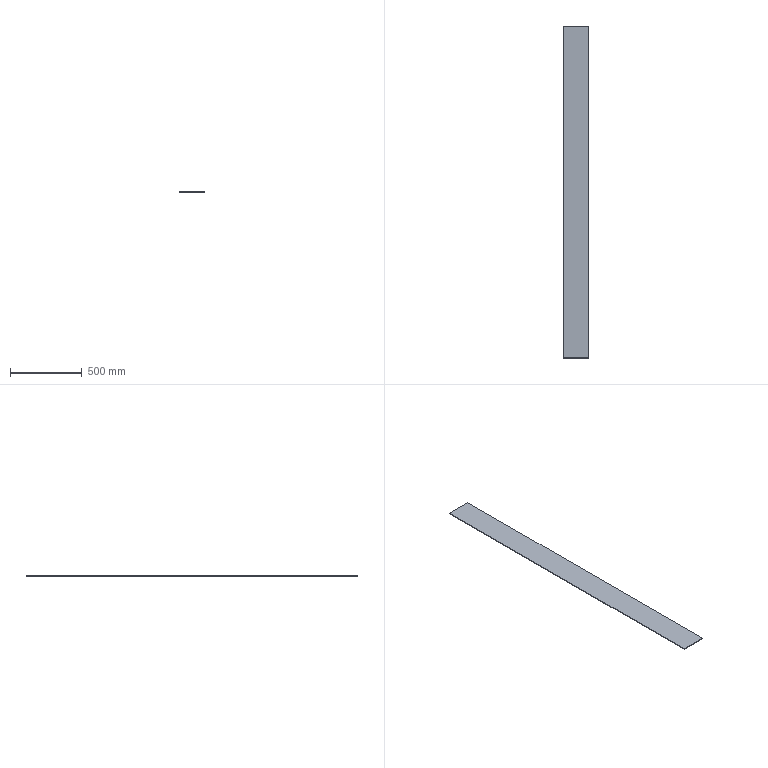Part | SolidWorks | features Extrusion 1, HoleWzd 1 | 1 solid | 6 faces | box 180 x 2310 x 5 mm | volume 2079000 mm3 | plane 6
STEP:
#1=CARTESIAN_POINT('',(90.,-1155.,0.));
#2=VERTEX_POINT('',#1);
#3=CARTESIAN_POINT('',(90.,1155.,0.));
#4=VERTEX_POINT('',#3);
#5=CARTESIAN_POINT('',(90.,1155.,0.));
#6=DIRECTION('',(0.,1.,0.));
#7=VECTOR('',#6,1000.);
#8=LINE('',#5,#7);
#9=EDGE_CURVE('',#2,#4,#8,.T.);
#10=ORIENTED_EDGE('',*,*,#9,.T.);
#11=CARTESIAN_POINT('',(90.,1155.,5.));
#12=VERTEX_POINT('',#11);
#13=CARTESIAN_POINT('',(90.,1155.,5.));
#14=DIRECTION('',(0.,0.,-1.));
#15=VECTOR('',#14,1000.);
#16=LINE('',#13,#15);
#17=EDGE_CURVE('',#12,#4,#16,.T.);
#18=ORIENTED_EDGE('',*,*,#17,.F.);
#19=CARTESIAN_POINT('',(90.,-1155.,5.));
#20=VERTEX_POINT('',#19);
#21=CARTESIAN_POINT('',(90.,1155.,5.));
#22=DIRECTION('',(0.,1.,0.));
#23=VECTOR('',#22,1000.);
#24=LINE('',#21,#23);
#25=EDGE_CURVE('',#20,#12,#24,.T.);
#26=ORIENTED_EDGE('',*,*,#25,.F.);
#27=CARTESIAN_POINT('',(90.,-1155.,5.));
#28=DIRECTION('',(0.,0.,-1.));
#29=VECTOR('',#28,1000.);
#30=LINE('',#27,#29);
#31=EDGE_CURVE('',#20,#2,#30,.T.);
#32=ORIENTED_EDGE('',*,*,#31,.T.);
#33=EDGE_LOOP('',(#10,#18,#26,#32));
#34=FACE_OUTER_BOUND('',#33,.T.);
#35=CARTESIAN_POINT('',(90.,1155.,5.));
#36=DIRECTION('',(-1.,0.,0.));
#37=DIRECTION('',(0.,-1.,0.));
#38=AXIS2_PLACEMENT_3D('',#35,#36,#37);
#39=PLANE('',#38);
#40=ADVANCED_FACE('',(#34),#39,.F.);
#41=CARTESIAN_POINT('',(-90.,1155.,0.));
#42=VERTEX_POINT('',#41);
#43=CARTESIAN_POINT('',(-90.,1155.,0.));
#44=DIRECTION('',(-1.,0.,0.));
#45=VECTOR('',#44,1000.);
#46=LINE('',#43,#45);
#47=EDGE_CURVE('',#4,#42,#46,.T.);
#48=ORIENTED_EDGE('',*,*,#47,.T.);
#49=CARTESIAN_POINT('',(-90.,1155.,5.));
#50=VERTEX_POINT('',#49);
#51=CARTESIAN_POINT('',(-90.,1155.,5.));
#52=DIRECTION('',(0.,0.,-1.));
#53=VECTOR('',#52,1000.);
#54=LINE('',#51,#53);
#55=EDGE_CURVE('',#50,#42,#54,.T.);
#56=ORIENTED_EDGE('',*,*,#55,.F.);
#57=CARTESIAN_POINT('',(-90.,1155.,5.));
#58=DIRECTION('',(-1.,0.,0.));
#59=VECTOR('',#58,1000.);
#60=LINE('',#57,#59);
#61=EDGE_CURVE('',#12,#50,#60,.T.);
#62=ORIENTED_EDGE('',*,*,#61,.F.);
#63=ORIENTED_EDGE('',*,*,#17,.T.);
#64=EDGE_LOOP('',(#48,#56,#62,#63));
#65=FACE_OUTER_BOUND('',#64,.T.);
#66=CARTESIAN_POINT('',(-90.,1155.,5.));
#67=DIRECTION('',(0.,-1.,0.));
#68=DIRECTION('',(0.,0.,-1.));
#69=AXIS2_PLACEMENT_3D('',#66,#67,#68);
#70=PLANE('',#69);
#71=ADVANCED_FACE('',(#65),#70,.F.);
#72=CARTESIAN_POINT('',(-90.,-1155.,0.));
#73=VERTEX_POINT('',#72);
#74=CARTESIAN_POINT('',(-90.,1155.,0.));
#75=DIRECTION('',(0.,-1.,0.));
#76=VECTOR('',#75,1000.);
#77=LINE('',#74,#76);
#78=EDGE_CURVE('',#42,#73,#77,.T.);
#79=ORIENTED_EDGE('',*,*,#78,.T.);
#80=CARTESIAN_POINT('',(-90.,-1155.,5.));
#81=VERTEX_POINT('',#80);
#82=CARTESIAN_POINT('',(-90.,-1155.,5.));
#83=DIRECTION('',(0.,0.,-1.));
#84=VECTOR('',#83,1000.);
#85=LINE('',#82,#84);
#86=EDGE_CURVE('',#81,#73,#85,.T.);
#87=ORIENTED_EDGE('',*,*,#86,.F.);
#88=CARTESIAN_POINT('',(-90.,1155.,5.));
#89=DIRECTION('',(0.,-1.,0.));
#90=VECTOR('',#89,1000.);
#91=LINE('',#88,#90);
#92=EDGE_CURVE('',#50,#81,#91,.T.);
#93=ORIENTED_EDGE('',*,*,#92,.F.);
#94=ORIENTED_EDGE('',*,*,#55,.T.);
#95=EDGE_LOOP('',(#79,#87,#93,#94));
#96=FACE_OUTER_BOUND('',#95,.T.);
#97=CARTESIAN_POINT('',(-90.,1155.,5.));
#98=DIRECTION('',(1.,0.,0.));
#99=DIRECTION('',(0.,1.,0.));
#100=AXIS2_PLACEMENT_3D('',#97,#98,#99);
#101=PLANE('',#100);
#102=ADVANCED_FACE('',(#96),#101,.F.);
#103=CARTESIAN_POINT('',(-90.,-1155.,0.));
#104=DIRECTION('',(1.,0.,0.));
#105=VECTOR('',#104,1000.);
#106=LINE('',#103,#105);
#107=EDGE_CURVE('',#73,#2,#106,.T.);
#108=ORIENTED_EDGE('',*,*,#107,.T.);
#109=ORIENTED_EDGE('',*,*,#31,.F.);
#110=CARTESIAN_POINT('',(-90.,-1155.,5.));
#111=DIRECTION('',(1.,0.,0.));
#112=VECTOR('',#111,1000.);
#113=LINE('',#110,#112);
#114=EDGE_CURVE('',#81,#20,#113,.T.);
#115=ORIENTED_EDGE('',*,*,#114,.F.);
#116=ORIENTED_EDGE('',*,*,#86,.T.);
#117=EDGE_LOOP('',(#108,#109,#115,#116));
#118=FACE_OUTER_BOUND('',#117,.T.);
#119=CARTESIAN_POINT('',(-90.,-1155.,5.));
#120=DIRECTION('',(0.,1.,0.));
#121=DIRECTION('',(0.,0.,1.));
#122=AXIS2_PLACEMENT_3D('',#119,#120,#121);
#123=PLANE('',#122);
#124=ADVANCED_FACE('',(#118),#123,.F.);
#125=ORIENTED_EDGE('',*,*,#25,.T.);
#126=ORIENTED_EDGE('',*,*,#61,.T.);
#127=ORIENTED_EDGE('',*,*,#92,.T.);
#128=ORIENTED_EDGE('',*,*,#114,.T.);
#129=EDGE_LOOP('',(#125,#126,#127,#128));
#130=FACE_OUTER_BOUND('',#129,.T.);
#131=CARTESIAN_POINT('',(0.,0.,5.));
#132=DIRECTION('',(0.,0.,1.));
#133=DIRECTION('',(1.,0.,0.));
#134=AXIS2_PLACEMENT_3D('',#131,#132,#133);
#135=PLANE('',#134);
#136=ADVANCED_FACE('',(#130),#135,.T.);
#137=ORIENTED_EDGE('',*,*,#9,.F.);
#138=ORIENTED_EDGE('',*,*,#107,.F.);
#139=ORIENTED_EDGE('',*,*,#78,.F.);
#140=ORIENTED_EDGE('',*,*,#47,.F.);
#141=EDGE_LOOP('',(#137,#138,#139,#140));
#142=FACE_OUTER_BOUND('',#141,.T.);
#143=CARTESIAN_POINT('',(0.,0.,0.));
#144=DIRECTION('',(0.,0.,1.));
#145=DIRECTION('',(1.,0.,0.));
#146=AXIS2_PLACEMENT_3D('',#143,#144,#145);
#147=PLANE('',#146);
#148=ADVANCED_FACE('',(#142),#147,.F.);
#149=CLOSED_SHELL('',(#40,#71,#102,#124,#136,#148));
#150=MANIFOLD_SOLID_BREP('',#149);
#151=CARTESIAN_POINT('',(0.,0.,0.));
#152=DIRECTION('',(0.,0.,1.));
#153=DIRECTION('',(1.,0.,0.));
#154=AXIS2_PLACEMENT_3D('',#151,#152,#153);
#155=(LENGTH_UNIT()NAMED_UNIT(*)SI_UNIT(.MILLI.,.METRE.));
#156=UNCERTAINTY_MEASURE_WITH_UNIT(LENGTH_MEASURE(0.00001),#155,'','');
#157=(NAMED_UNIT(*)PLANE_ANGLE_UNIT()SI_UNIT($,.RADIAN.));
#158=(NAMED_UNIT(*)SI_UNIT($,.STERADIAN.)SOLID_ANGLE_UNIT());
#159=(GEOMETRIC_REPRESENTATION_CONTEXT(3)GLOBAL_UNCERTAINTY_ASSIGNED_CONTEXT((#156))GLOBAL_UNIT_ASSIGNED_CONTEXT((#155,#157,#158))REPRESENTATION_CONTEXT('',''));
#160=ADVANCED_BREP_SHAPE_REPRESENTATION('',(#150,#154),#159);